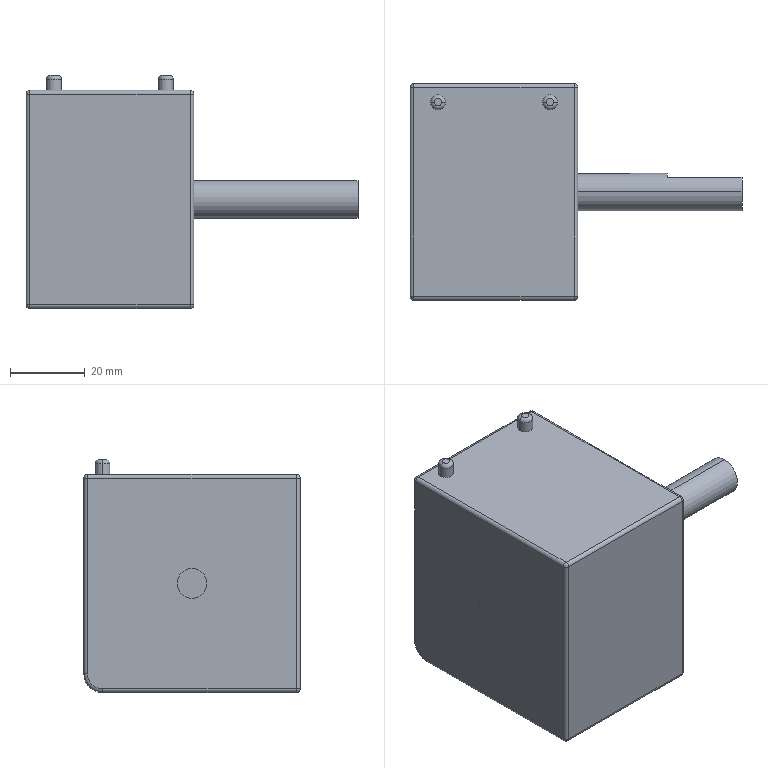Part | STEP file | MJ45 motor support seat | 1 solid | 224 faces | box 89 x 58 x 62.5 mm | volume 152707 mm3 | plane 90 | cylinder 78 | torus 42 | cone 8 | sphere 6 | commonest cylinder face diameters 2 x56 4.2 x8 5.5 x6 4 x4 10 x4